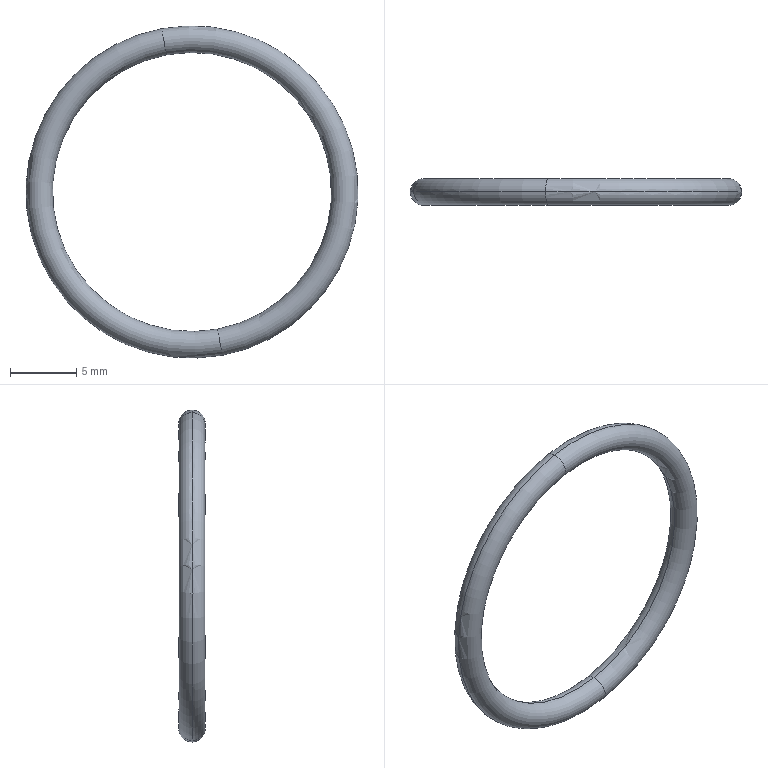Part | SolidWorks | features BaseBody 1 | 1 solid | 4 faces | box 25 x 2 x 25 mm | volume 227.001 mm3 | torus 4
STEP:
#1=CARTESIAN_POINT('',(34.219,180.1,12.29));
#2=VERTEX_POINT('',#1);
#3=CARTESIAN_POINT('',(34.584,180.1,10.324));
#4=VERTEX_POINT('',#3);
#5=CARTESIAN_POINT('',(34.401,180.1,11.307));
#6=DIRECTION('',(0.9832,0.,0.1825));
#7=DIRECTION('',(0.1825,0.,-0.9832));
#8=AXIS2_PLACEMENT_3D('',#5,#6,#7);
#9=CIRCLE('',#8,1.);
#10=EDGE_CURVE('',#2,#4,#9,.T.);
#11=ORIENTED_EDGE('',*,*,#10,.F.);
#12=CARTESIAN_POINT('',(38.781,180.1,-12.29));
#13=VERTEX_POINT('',#12);
#14=CARTESIAN_POINT('',(36.5,180.1,0.));
#15=DIRECTION('',(0.,-1.,0.));
#16=DIRECTION('',(0.,0.,-1.));
#17=AXIS2_PLACEMENT_3D('',#14,#15,#16);
#18=CIRCLE('',#17,12.5);
#19=EDGE_CURVE('',#2,#13,#18,.T.);
#20=ORIENTED_EDGE('',*,*,#19,.T.);
#21=CARTESIAN_POINT('',(38.416,180.1,-10.324));
#22=VERTEX_POINT('',#21);
#23=CARTESIAN_POINT('',(38.599,180.1,-11.307));
#24=DIRECTION('',(-0.9832,0.,-0.1825));
#25=DIRECTION('',(-0.1825,0.,0.9832));
#26=AXIS2_PLACEMENT_3D('',#23,#24,#25);
#27=CIRCLE('',#26,1.);
#28=EDGE_CURVE('',#13,#22,#27,.T.);
#29=ORIENTED_EDGE('',*,*,#28,.T.);
#30=CARTESIAN_POINT('',(36.5,180.1,0.));
#31=DIRECTION('',(0.,-1.,0.));
#32=DIRECTION('',(0.,0.,-1.));
#33=AXIS2_PLACEMENT_3D('',#30,#31,#32);
#34=CIRCLE('',#33,10.5);
#35=EDGE_CURVE('',#4,#22,#34,.T.);
#36=ORIENTED_EDGE('',*,*,#35,.F.);
#37=EDGE_LOOP('',(#11,#20,#29,#36));
#38=FACE_OUTER_BOUND('',#37,.T.);
#39=CARTESIAN_POINT('',(36.5,180.1,0.));
#40=DIRECTION('',(0.,-1.,0.));
#41=DIRECTION('',(0.1825,0.,-0.9832));
#42=AXIS2_PLACEMENT_3D('',#39,#40,#41);
#43=TOROIDAL_SURFACE('',#42,11.5,1.);
#44=ADVANCED_FACE('',(#38),#43,.T.);
#45=ORIENTED_EDGE('',*,*,#28,.F.);
#46=CARTESIAN_POINT('',(36.5,180.1,0.));
#47=DIRECTION('',(0.,-1.,0.));
#48=DIRECTION('',(0.,0.,-1.));
#49=AXIS2_PLACEMENT_3D('',#46,#47,#48);
#50=CIRCLE('',#49,12.5);
#51=EDGE_CURVE('',#13,#2,#50,.T.);
#52=ORIENTED_EDGE('',*,*,#51,.T.);
#53=ORIENTED_EDGE('',*,*,#10,.T.);
#54=CARTESIAN_POINT('',(36.5,180.1,0.));
#55=DIRECTION('',(0.,-1.,0.));
#56=DIRECTION('',(0.,0.,-1.));
#57=AXIS2_PLACEMENT_3D('',#54,#55,#56);
#58=CIRCLE('',#57,10.5);
#59=EDGE_CURVE('',#22,#4,#58,.T.);
#60=ORIENTED_EDGE('',*,*,#59,.F.);
#61=EDGE_LOOP('',(#45,#52,#53,#60));
#62=FACE_OUTER_BOUND('',#61,.T.);
#63=CARTESIAN_POINT('',(36.5,180.1,0.));
#64=DIRECTION('',(0.,-1.,0.));
#65=DIRECTION('',(0.1825,0.,-0.9832));
#66=AXIS2_PLACEMENT_3D('',#63,#64,#65);
#67=TOROIDAL_SURFACE('',#66,11.5,1.);
#68=ADVANCED_FACE('',(#62),#67,.T.);
#69=ORIENTED_EDGE('',*,*,#51,.F.);
#70=CARTESIAN_POINT('',(38.599,180.1,-11.307));
#71=DIRECTION('',(-0.9832,0.,-0.1825));
#72=DIRECTION('',(-0.1825,0.,0.9832));
#73=AXIS2_PLACEMENT_3D('',#70,#71,#72);
#74=CIRCLE('',#73,1.);
#75=EDGE_CURVE('',#22,#13,#74,.T.);
#76=ORIENTED_EDGE('',*,*,#75,.F.);
#77=ORIENTED_EDGE('',*,*,#59,.T.);
#78=CARTESIAN_POINT('',(34.401,180.1,11.307));
#79=DIRECTION('',(0.9832,0.,0.1825));
#80=DIRECTION('',(0.1825,0.,-0.9832));
#81=AXIS2_PLACEMENT_3D('',#78,#79,#80);
#82=CIRCLE('',#81,1.);
#83=EDGE_CURVE('',#4,#2,#82,.T.);
#84=ORIENTED_EDGE('',*,*,#83,.T.);
#85=EDGE_LOOP('',(#69,#76,#77,#84));
#86=FACE_OUTER_BOUND('',#85,.T.);
#87=CARTESIAN_POINT('',(36.5,180.1,0.));
#88=DIRECTION('',(0.,-1.,0.));
#89=DIRECTION('',(0.1825,0.,-0.9832));
#90=AXIS2_PLACEMENT_3D('',#87,#88,#89);
#91=TOROIDAL_SURFACE('',#90,11.5,1.);
#92=ADVANCED_FACE('',(#86),#91,.T.);
#93=ORIENTED_EDGE('',*,*,#19,.F.);
#94=ORIENTED_EDGE('',*,*,#83,.F.);
#95=ORIENTED_EDGE('',*,*,#35,.T.);
#96=ORIENTED_EDGE('',*,*,#75,.T.);
#97=EDGE_LOOP('',(#93,#94,#95,#96));
#98=FACE_OUTER_BOUND('',#97,.T.);
#99=CARTESIAN_POINT('',(36.5,180.1,0.));
#100=DIRECTION('',(0.,-1.,0.));
#101=DIRECTION('',(0.1825,0.,-0.9832));
#102=AXIS2_PLACEMENT_3D('',#99,#100,#101);
#103=TOROIDAL_SURFACE('',#102,11.5,1.);
#104=ADVANCED_FACE('',(#98),#103,.T.);
#105=CLOSED_SHELL('',(#44,#68,#92,#104));
#106=MANIFOLD_SOLID_BREP('',#105);
#107=CARTESIAN_POINT('',(0.,0.,0.));
#108=DIRECTION('',(0.,0.,1.));
#109=DIRECTION('',(1.,0.,0.));
#110=AXIS2_PLACEMENT_3D('',#107,#108,#109);
#111=(LENGTH_UNIT()NAMED_UNIT(*)SI_UNIT(.MILLI.,.METRE.));
#112=UNCERTAINTY_MEASURE_WITH_UNIT(LENGTH_MEASURE(0.00001),#111,'','');
#113=(NAMED_UNIT(*)PLANE_ANGLE_UNIT()SI_UNIT($,.RADIAN.));
#114=(NAMED_UNIT(*)SI_UNIT($,.STERADIAN.)SOLID_ANGLE_UNIT());
#115=(GEOMETRIC_REPRESENTATION_CONTEXT(3)GLOBAL_UNCERTAINTY_ASSIGNED_CONTEXT((#112))GLOBAL_UNIT_ASSIGNED_CONTEXT((#111,#113,#114))REPRESENTATION_CONTEXT('',''));
#116=ADVANCED_BREP_SHAPE_REPRESENTATION('',(#106,#110),#115);